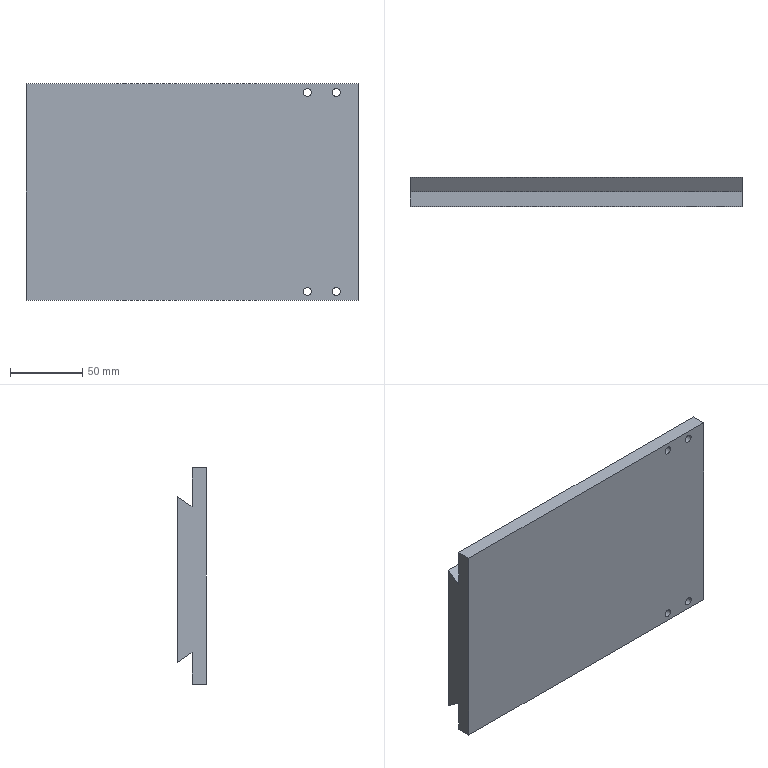Part | STEP file | 06-29 Up-down adjusting dovetail plate | 1 solid | 38 faces | box 230 x 20 x 150 mm | volume 590829 mm3 | cylinder 20 | plane 14 | cone 4 | commonest cylinder face diameters 5.5 x8 10 x8 4.2 x4